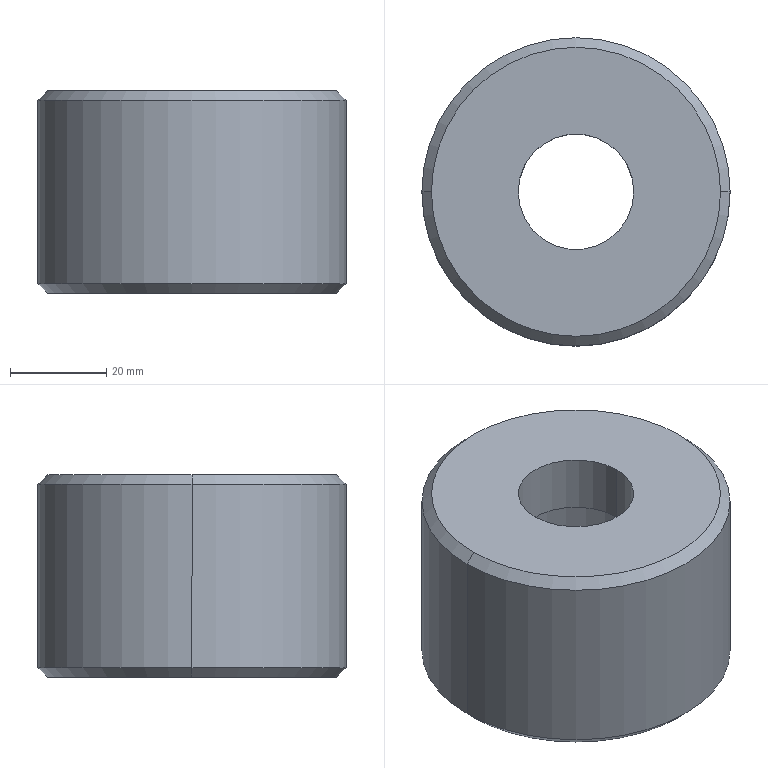Part | SolidWorks | features BaseBody 1 | 1 solid | 13 faces | box 64 x 64 x 42 mm | volume 76849 mm3 | cylinder 6 | cone 4 | plane 3 | commonest cylinder face diameters 24 x2 47 x2 64 x2
STEP:
#1=CARTESIAN_POINT('',(-32.,0.,-2.));
#2=VERTEX_POINT('',#1);
#3=CARTESIAN_POINT('',(32.,0.,-2.));
#4=VERTEX_POINT('',#3);
#5=CARTESIAN_POINT('',(0.,0.,-2.));
#6=DIRECTION('',(0.,0.,-1.));
#7=DIRECTION('',(-1.,0.,0.));
#8=AXIS2_PLACEMENT_3D('',#5,#6,#7);
#9=CIRCLE('',#8,32.);
#10=EDGE_CURVE('',#2,#4,#9,.T.);
#11=ORIENTED_EDGE('',*,*,#10,.T.);
#12=CARTESIAN_POINT('',(32.,0.,-40.));
#13=VERTEX_POINT('',#12);
#14=CARTESIAN_POINT('',(32.,0.,-21.));
#15=DIRECTION('',(0.,0.,-1.));
#16=VECTOR('',#15,1000.);
#17=LINE('',#14,#16);
#18=EDGE_CURVE('',#4,#13,#17,.T.);
#19=ORIENTED_EDGE('',*,*,#18,.T.);
#20=CARTESIAN_POINT('',(-32.,0.,-40.));
#21=VERTEX_POINT('',#20);
#22=CARTESIAN_POINT('',(0.,0.,-40.));
#23=DIRECTION('',(0.,0.,1.));
#24=DIRECTION('',(-1.,0.,0.));
#25=AXIS2_PLACEMENT_3D('',#22,#23,#24);
#26=CIRCLE('',#25,32.);
#27=EDGE_CURVE('',#13,#21,#26,.T.);
#28=ORIENTED_EDGE('',*,*,#27,.T.);
#29=CARTESIAN_POINT('',(-32.,0.,-21.));
#30=DIRECTION('',(0.,0.,-1.));
#31=VECTOR('',#30,1000.);
#32=LINE('',#29,#31);
#33=EDGE_CURVE('',#2,#21,#32,.T.);
#34=ORIENTED_EDGE('',*,*,#33,.F.);
#35=EDGE_LOOP('',(#11,#19,#28,#34));
#36=FACE_OUTER_BOUND('',#35,.T.);
#37=CARTESIAN_POINT('',(0.,0.,-21.));
#38=DIRECTION('',(0.,0.,-1.));
#39=DIRECTION('',(-1.,0.,0.));
#40=AXIS2_PLACEMENT_3D('',#37,#38,#39);
#41=CYLINDRICAL_SURFACE('',#40,32.);
#42=ADVANCED_FACE('',(#36),#41,.T.);
#43=CARTESIAN_POINT('',(30.,0.,-42.));
#44=VERTEX_POINT('',#43);
#45=CARTESIAN_POINT('',(-30.,0.,-42.));
#46=VERTEX_POINT('',#45);
#47=CARTESIAN_POINT('',(0.,0.,-42.));
#48=DIRECTION('',(0.,0.,1.));
#49=DIRECTION('',(1.,0.,0.));
#50=AXIS2_PLACEMENT_3D('',#47,#48,#49);
#51=CIRCLE('',#50,30.);
#52=EDGE_CURVE('',#44,#46,#51,.T.);
#53=ORIENTED_EDGE('',*,*,#52,.T.);
#54=CARTESIAN_POINT('',(-32.,0.,-40.));
#55=DIRECTION('',(-0.7071,0.,0.7071));
#56=VECTOR('',#55,1000.);
#57=LINE('',#54,#56);
#58=EDGE_CURVE('',#46,#21,#57,.T.);
#59=ORIENTED_EDGE('',*,*,#58,.T.);
#60=ORIENTED_EDGE('',*,*,#27,.F.);
#61=CARTESIAN_POINT('',(32.,0.,-40.));
#62=DIRECTION('',(0.7071,0.,0.7071));
#63=VECTOR('',#62,1000.);
#64=LINE('',#61,#63);
#65=EDGE_CURVE('',#44,#13,#64,.T.);
#66=ORIENTED_EDGE('',*,*,#65,.F.);
#67=EDGE_LOOP('',(#53,#59,#60,#66));
#68=FACE_OUTER_BOUND('',#67,.T.);
#69=CARTESIAN_POINT('',(0.,0.,-40.));
#70=DIRECTION('',(0.,0.,1.));
#71=DIRECTION('',(1.,0.,0.));
#72=AXIS2_PLACEMENT_3D('',#69,#70,#71);
#73=CONICAL_SURFACE('',#72,32.,0.7854);
#74=ADVANCED_FACE('',(#68),#73,.T.);
#75=CARTESIAN_POINT('',(-30.,0.,0.));
#76=VERTEX_POINT('',#75);
#77=CARTESIAN_POINT('',(30.,0.,0.));
#78=VERTEX_POINT('',#77);
#79=CARTESIAN_POINT('',(0.,0.,0.));
#80=DIRECTION('',(0.,0.,-1.));
#81=DIRECTION('',(-1.,0.,0.));
#82=AXIS2_PLACEMENT_3D('',#79,#80,#81);
#83=CIRCLE('',#82,30.);
#84=EDGE_CURVE('',#76,#78,#83,.T.);
#85=ORIENTED_EDGE('',*,*,#84,.T.);
#86=CARTESIAN_POINT('',(32.,0.,-2.));
#87=DIRECTION('',(0.7071,0.,-0.7071));
#88=VECTOR('',#87,1000.);
#89=LINE('',#86,#88);
#90=EDGE_CURVE('',#78,#4,#89,.T.);
#91=ORIENTED_EDGE('',*,*,#90,.T.);
#92=ORIENTED_EDGE('',*,*,#10,.F.);
#93=CARTESIAN_POINT('',(-32.,0.,-2.));
#94=DIRECTION('',(-0.7071,0.,-0.7071));
#95=VECTOR('',#94,1000.);
#96=LINE('',#93,#95);
#97=EDGE_CURVE('',#76,#2,#96,.T.);
#98=ORIENTED_EDGE('',*,*,#97,.F.);
#99=EDGE_LOOP('',(#85,#91,#92,#98));
#100=FACE_OUTER_BOUND('',#99,.T.);
#101=CARTESIAN_POINT('',(0.,0.,-2.));
#102=DIRECTION('',(0.,0.,-1.));
#103=DIRECTION('',(-1.,0.,0.));
#104=AXIS2_PLACEMENT_3D('',#101,#102,#103);
#105=CONICAL_SURFACE('',#104,32.,0.7854);
#106=ADVANCED_FACE('',(#100),#105,.T.);
#107=CARTESIAN_POINT('',(23.5,0.,-12.));
#108=VERTEX_POINT('',#107);
#109=CARTESIAN_POINT('',(-23.5,0.,-12.));
#110=VERTEX_POINT('',#109);
#111=CARTESIAN_POINT('',(0.,0.,-12.));
#112=DIRECTION('',(0.,0.,-1.));
#113=DIRECTION('',(-1.,0.,0.));
#114=AXIS2_PLACEMENT_3D('',#111,#112,#113);
#115=CIRCLE('',#114,23.5);
#116=EDGE_CURVE('',#108,#110,#115,.T.);
#117=ORIENTED_EDGE('',*,*,#116,.F.);
#118=CARTESIAN_POINT('',(23.5,0.,-42.));
#119=VERTEX_POINT('',#118);
#120=CARTESIAN_POINT('',(23.5,0.,-27.));
#121=DIRECTION('',(0.,0.,-1.));
#122=VECTOR('',#121,1000.);
#123=LINE('',#120,#122);
#124=EDGE_CURVE('',#108,#119,#123,.T.);
#125=ORIENTED_EDGE('',*,*,#124,.T.);
#126=CARTESIAN_POINT('',(-23.5,0.,-42.));
#127=VERTEX_POINT('',#126);
#128=CARTESIAN_POINT('',(0.,0.,-42.));
#129=DIRECTION('',(0.,0.,1.));
#130=DIRECTION('',(-1.,0.,0.));
#131=AXIS2_PLACEMENT_3D('',#128,#129,#130);
#132=CIRCLE('',#131,23.5);
#133=EDGE_CURVE('',#127,#119,#132,.T.);
#134=ORIENTED_EDGE('',*,*,#133,.F.);
#135=CARTESIAN_POINT('',(-23.5,0.,-27.));
#136=DIRECTION('',(0.,0.,-1.));
#137=VECTOR('',#136,1000.);
#138=LINE('',#135,#137);
#139=EDGE_CURVE('',#110,#127,#138,.T.);
#140=ORIENTED_EDGE('',*,*,#139,.F.);
#141=EDGE_LOOP('',(#117,#125,#134,#140));
#142=FACE_OUTER_BOUND('',#141,.T.);
#143=CARTESIAN_POINT('',(0.,0.,-27.));
#144=DIRECTION('',(0.,0.,-1.));
#145=DIRECTION('',(-1.,0.,0.));
#146=AXIS2_PLACEMENT_3D('',#143,#144,#145);
#147=CYLINDRICAL_SURFACE('',#146,23.5);
#148=ADVANCED_FACE('',(#142),#147,.F.);
#149=CARTESIAN_POINT('',(12.,0.,0.));
#150=VERTEX_POINT('',#149);
#151=CARTESIAN_POINT('',(-12.,0.,0.));
#152=VERTEX_POINT('',#151);
#153=CARTESIAN_POINT('',(0.,0.,0.));
#154=DIRECTION('',(0.,0.,-1.));
#155=DIRECTION('',(-1.,0.,0.));
#156=AXIS2_PLACEMENT_3D('',#153,#154,#155);
#157=CIRCLE('',#156,12.);
#158=EDGE_CURVE('',#150,#152,#157,.T.);
#159=ORIENTED_EDGE('',*,*,#158,.F.);
#160=CARTESIAN_POINT('',(12.,0.,-12.));
#161=VERTEX_POINT('',#160);
#162=CARTESIAN_POINT('',(12.,0.,-6.));
#163=DIRECTION('',(0.,0.,-1.));
#164=VECTOR('',#163,1000.);
#165=LINE('',#162,#164);
#166=EDGE_CURVE('',#150,#161,#165,.T.);
#167=ORIENTED_EDGE('',*,*,#166,.T.);
#168=CARTESIAN_POINT('',(-12.,0.,-12.));
#169=VERTEX_POINT('',#168);
#170=CARTESIAN_POINT('',(0.,0.,-12.));
#171=DIRECTION('',(0.,0.,1.));
#172=DIRECTION('',(-1.,0.,0.));
#173=AXIS2_PLACEMENT_3D('',#170,#171,#172);
#174=CIRCLE('',#173,12.);
#175=EDGE_CURVE('',#169,#161,#174,.T.);
#176=ORIENTED_EDGE('',*,*,#175,.F.);
#177=CARTESIAN_POINT('',(-12.,0.,-6.));
#178=DIRECTION('',(0.,0.,-1.));
#179=VECTOR('',#178,1000.);
#180=LINE('',#177,#179);
#181=EDGE_CURVE('',#152,#169,#180,.T.);
#182=ORIENTED_EDGE('',*,*,#181,.F.);
#183=EDGE_LOOP('',(#159,#167,#176,#182));
#184=FACE_OUTER_BOUND('',#183,.T.);
#185=CARTESIAN_POINT('',(0.,0.,-6.));
#186=DIRECTION('',(0.,0.,-1.));
#187=DIRECTION('',(-1.,0.,0.));
#188=AXIS2_PLACEMENT_3D('',#185,#186,#187);
#189=CYLINDRICAL_SURFACE('',#188,12.);
#190=ADVANCED_FACE('',(#184),#189,.F.);
#191=ORIENTED_EDGE('',*,*,#18,.F.);
#192=CARTESIAN_POINT('',(0.,0.,-2.));
#193=DIRECTION('',(0.,0.,-1.));
#194=DIRECTION('',(-1.,0.,0.));
#195=AXIS2_PLACEMENT_3D('',#192,#193,#194);
#196=CIRCLE('',#195,32.);
#197=EDGE_CURVE('',#4,#2,#196,.T.);
#198=ORIENTED_EDGE('',*,*,#197,.T.);
#199=ORIENTED_EDGE('',*,*,#33,.T.);
#200=CARTESIAN_POINT('',(0.,0.,-40.));
#201=DIRECTION('',(0.,0.,1.));
#202=DIRECTION('',(-1.,0.,0.));
#203=AXIS2_PLACEMENT_3D('',#200,#201,#202);
#204=CIRCLE('',#203,32.);
#205=EDGE_CURVE('',#21,#13,#204,.T.);
#206=ORIENTED_EDGE('',*,*,#205,.T.);
#207=EDGE_LOOP('',(#191,#198,#199,#206));
#208=FACE_OUTER_BOUND('',#207,.T.);
#209=CARTESIAN_POINT('',(0.,0.,-21.));
#210=DIRECTION('',(0.,0.,-1.));
#211=DIRECTION('',(-1.,0.,0.));
#212=AXIS2_PLACEMENT_3D('',#209,#210,#211);
#213=CYLINDRICAL_SURFACE('',#212,32.);
#214=ADVANCED_FACE('',(#208),#213,.T.);
#215=ORIENTED_EDGE('',*,*,#58,.F.);
#216=CARTESIAN_POINT('',(0.,0.,-42.));
#217=DIRECTION('',(0.,0.,1.));
#218=DIRECTION('',(1.,0.,0.));
#219=AXIS2_PLACEMENT_3D('',#216,#217,#218);
#220=CIRCLE('',#219,30.);
#221=EDGE_CURVE('',#46,#44,#220,.T.);
#222=ORIENTED_EDGE('',*,*,#221,.T.);
#223=ORIENTED_EDGE('',*,*,#65,.T.);
#224=ORIENTED_EDGE('',*,*,#205,.F.);
#225=EDGE_LOOP('',(#215,#222,#223,#224));
#226=FACE_OUTER_BOUND('',#225,.T.);
#227=CARTESIAN_POINT('',(0.,0.,-40.));
#228=DIRECTION('',(0.,0.,1.));
#229=DIRECTION('',(1.,0.,0.));
#230=AXIS2_PLACEMENT_3D('',#227,#228,#229);
#231=CONICAL_SURFACE('',#230,32.,0.7854);
#232=ADVANCED_FACE('',(#226),#231,.T.);
#233=ORIENTED_EDGE('',*,*,#90,.F.);
#234=CARTESIAN_POINT('',(0.,0.,0.));
#235=DIRECTION('',(0.,0.,-1.));
#236=DIRECTION('',(-1.,0.,0.));
#237=AXIS2_PLACEMENT_3D('',#234,#235,#236);
#238=CIRCLE('',#237,30.);
#239=EDGE_CURVE('',#78,#76,#238,.T.);
#240=ORIENTED_EDGE('',*,*,#239,.T.);
#241=ORIENTED_EDGE('',*,*,#97,.T.);
#242=ORIENTED_EDGE('',*,*,#197,.F.);
#243=EDGE_LOOP('',(#233,#240,#241,#242));
#244=FACE_OUTER_BOUND('',#243,.T.);
#245=CARTESIAN_POINT('',(0.,0.,-2.));
#246=DIRECTION('',(0.,0.,-1.));
#247=DIRECTION('',(-1.,0.,0.));
#248=AXIS2_PLACEMENT_3D('',#245,#246,#247);
#249=CONICAL_SURFACE('',#248,32.,0.7854);
#250=ADVANCED_FACE('',(#244),#249,.T.);
#251=ORIENTED_EDGE('',*,*,#133,.T.);
#252=CARTESIAN_POINT('',(0.,0.,-42.));
#253=DIRECTION('',(0.,0.,1.));
#254=DIRECTION('',(-1.,0.,0.));
#255=AXIS2_PLACEMENT_3D('',#252,#253,#254);
#256=CIRCLE('',#255,23.5);
#257=EDGE_CURVE('',#119,#127,#256,.T.);
#258=ORIENTED_EDGE('',*,*,#257,.T.);
#259=EDGE_LOOP('',(#251,#258));
#260=FACE_BOUND('',#259,.T.);
#261=ORIENTED_EDGE('',*,*,#52,.F.);
#262=ORIENTED_EDGE('',*,*,#221,.F.);
#263=EDGE_LOOP('',(#261,#262));
#264=FACE_OUTER_BOUND('',#263,.T.);
#265=CARTESIAN_POINT('',(-23.5,0.,-42.));
#266=DIRECTION('',(0.,0.,-1.));
#267=DIRECTION('',(-1.,0.,0.));
#268=AXIS2_PLACEMENT_3D('',#265,#266,#267);
#269=PLANE('',#268);
#270=ADVANCED_FACE('',(#260,#264),#269,.T.);
#271=CARTESIAN_POINT('',(0.,0.,0.));
#272=DIRECTION('',(0.,0.,-1.));
#273=DIRECTION('',(-1.,0.,0.));
#274=AXIS2_PLACEMENT_3D('',#271,#272,#273);
#275=CIRCLE('',#274,12.);
#276=EDGE_CURVE('',#152,#150,#275,.T.);
#277=ORIENTED_EDGE('',*,*,#276,.T.);
#278=ORIENTED_EDGE('',*,*,#158,.T.);
#279=EDGE_LOOP('',(#277,#278));
#280=FACE_BOUND('',#279,.T.);
#281=ORIENTED_EDGE('',*,*,#84,.F.);
#282=ORIENTED_EDGE('',*,*,#239,.F.);
#283=EDGE_LOOP('',(#281,#282));
#284=FACE_OUTER_BOUND('',#283,.T.);
#285=CARTESIAN_POINT('',(-32.,0.,0.));
#286=DIRECTION('',(0.,0.,1.));
#287=DIRECTION('',(1.,0.,0.));
#288=AXIS2_PLACEMENT_3D('',#285,#286,#287);
#289=PLANE('',#288);
#290=ADVANCED_FACE('',(#280,#284),#289,.T.);
#291=ORIENTED_EDGE('',*,*,#124,.F.);
#292=CARTESIAN_POINT('',(0.,0.,-12.));
#293=DIRECTION('',(0.,0.,-1.));
#294=DIRECTION('',(-1.,0.,0.));
#295=AXIS2_PLACEMENT_3D('',#292,#293,#294);
#296=CIRCLE('',#295,23.5);
#297=EDGE_CURVE('',#110,#108,#296,.T.);
#298=ORIENTED_EDGE('',*,*,#297,.F.);
#299=ORIENTED_EDGE('',*,*,#139,.T.);
#300=ORIENTED_EDGE('',*,*,#257,.F.);
#301=EDGE_LOOP('',(#291,#298,#299,#300));
#302=FACE_OUTER_BOUND('',#301,.T.);
#303=CARTESIAN_POINT('',(0.,0.,-27.));
#304=DIRECTION('',(0.,0.,-1.));
#305=DIRECTION('',(-1.,0.,0.));
#306=AXIS2_PLACEMENT_3D('',#303,#304,#305);
#307=CYLINDRICAL_SURFACE('',#306,23.5);
#308=ADVANCED_FACE('',(#302),#307,.F.);
#309=ORIENTED_EDGE('',*,*,#166,.F.);
#310=ORIENTED_EDGE('',*,*,#276,.F.);
#311=ORIENTED_EDGE('',*,*,#181,.T.);
#312=CARTESIAN_POINT('',(0.,0.,-12.));
#313=DIRECTION('',(0.,0.,1.));
#314=DIRECTION('',(-1.,0.,0.));
#315=AXIS2_PLACEMENT_3D('',#312,#313,#314);
#316=CIRCLE('',#315,12.);
#317=EDGE_CURVE('',#161,#169,#316,.T.);
#318=ORIENTED_EDGE('',*,*,#317,.F.);
#319=EDGE_LOOP('',(#309,#310,#311,#318));
#320=FACE_OUTER_BOUND('',#319,.T.);
#321=CARTESIAN_POINT('',(0.,0.,-6.));
#322=DIRECTION('',(0.,0.,-1.));
#323=DIRECTION('',(-1.,0.,0.));
#324=AXIS2_PLACEMENT_3D('',#321,#322,#323);
#325=CYLINDRICAL_SURFACE('',#324,12.);
#326=ADVANCED_FACE('',(#320),#325,.F.);
#327=ORIENTED_EDGE('',*,*,#175,.T.);
#328=ORIENTED_EDGE('',*,*,#317,.T.);
#329=EDGE_LOOP('',(#327,#328));
#330=FACE_BOUND('',#329,.T.);
#331=ORIENTED_EDGE('',*,*,#297,.T.);
#332=ORIENTED_EDGE('',*,*,#116,.T.);
#333=EDGE_LOOP('',(#331,#332));
#334=FACE_OUTER_BOUND('',#333,.T.);
#335=CARTESIAN_POINT('',(-12.,0.,-12.));
#336=DIRECTION('',(0.,0.,-1.));
#337=DIRECTION('',(-1.,0.,0.));
#338=AXIS2_PLACEMENT_3D('',#335,#336,#337);
#339=PLANE('',#338);
#340=ADVANCED_FACE('',(#330,#334),#339,.T.);
#341=CLOSED_SHELL('',(#42,#74,#106,#148,#190,#214,#232,#250,#270,#290,#308,#326,#340));
#342=MANIFOLD_SOLID_BREP('',#341);
#343=CARTESIAN_POINT('',(0.,0.,0.));
#344=DIRECTION('',(0.,0.,1.));
#345=DIRECTION('',(1.,0.,0.));
#346=AXIS2_PLACEMENT_3D('',#343,#344,#345);
#347=(LENGTH_UNIT()NAMED_UNIT(*)SI_UNIT(.MILLI.,.METRE.));
#348=UNCERTAINTY_MEASURE_WITH_UNIT(LENGTH_MEASURE(0.00001),#347,'','');
#349=(NAMED_UNIT(*)PLANE_ANGLE_UNIT()SI_UNIT($,.RADIAN.));
#350=(NAMED_UNIT(*)SI_UNIT($,.STERADIAN.)SOLID_ANGLE_UNIT());
#351=(GEOMETRIC_REPRESENTATION_CONTEXT(3)GLOBAL_UNCERTAINTY_ASSIGNED_CONTEXT((#348))GLOBAL_UNIT_ASSIGNED_CONTEXT((#347,#349,#350))REPRESENTATION_CONTEXT('',''));
#352=ADVANCED_BREP_SHAPE_REPRESENTATION('',(#342,#346),#351);